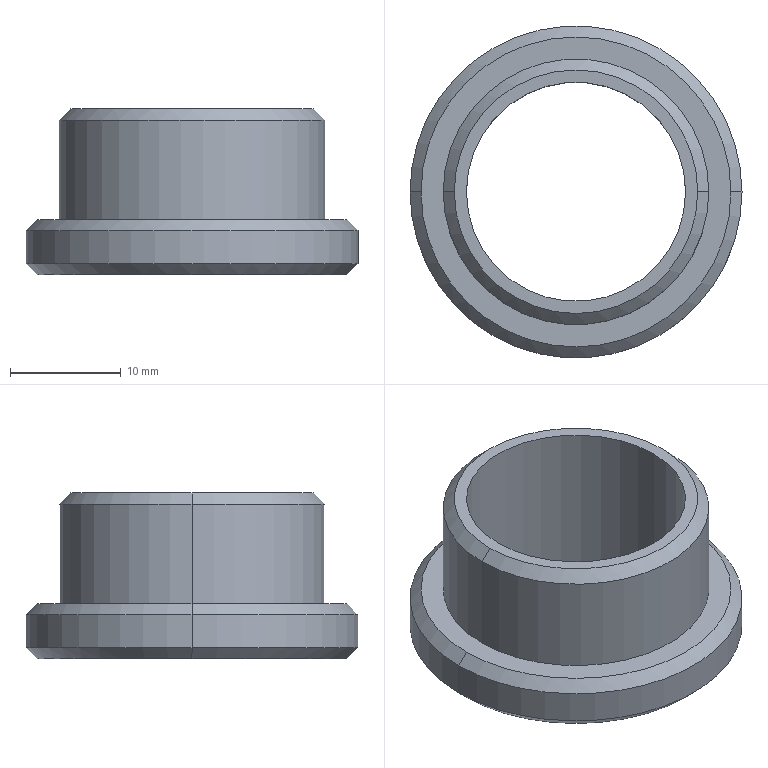Part | SolidWorks | features Chamfer 1, Extrusion 1, ICE 1 | 1 solid | 15 faces | box 30 x 30 x 15 mm | volume 3311 mm3 | cone 6 | cylinder 6 | plane 3 | commonest cylinder face diameters 19.8 x2 24 x2 30 x2
STEP:
#1=CARTESIAN_POINT('',(14.,0.,5.));
#2=VERTEX_POINT('',#1);
#3=CARTESIAN_POINT('',(-14.,0.,5.));
#4=VERTEX_POINT('',#3);
#5=CARTESIAN_POINT('',(0.,0.,5.));
#6=DIRECTION('',(0.,0.,1.));
#7=DIRECTION('',(1.,0.,0.));
#8=AXIS2_PLACEMENT_3D('',#5,#6,#7);
#9=CIRCLE('',#8,14.);
#10=EDGE_CURVE('',#2,#4,#9,.T.);
#11=ORIENTED_EDGE('',*,*,#10,.F.);
#12=CARTESIAN_POINT('',(15.,0.,4.));
#13=VERTEX_POINT('',#12);
#14=CARTESIAN_POINT('',(14.,0.,5.));
#15=DIRECTION('',(0.7071,0.,-0.7071));
#16=VECTOR('',#15,1000.);
#17=LINE('',#14,#16);
#18=EDGE_CURVE('',#2,#13,#17,.T.);
#19=ORIENTED_EDGE('',*,*,#18,.T.);
#20=CARTESIAN_POINT('',(-15.,0.,4.));
#21=VERTEX_POINT('',#20);
#22=CARTESIAN_POINT('',(0.,0.,4.));
#23=DIRECTION('',(0.,0.,-1.));
#24=DIRECTION('',(1.,0.,0.));
#25=AXIS2_PLACEMENT_3D('',#22,#23,#24);
#26=CIRCLE('',#25,15.);
#27=EDGE_CURVE('',#21,#13,#26,.T.);
#28=ORIENTED_EDGE('',*,*,#27,.F.);
#29=CARTESIAN_POINT('',(-14.,0.,5.));
#30=DIRECTION('',(-0.7071,0.,-0.7071));
#31=VECTOR('',#30,1000.);
#32=LINE('',#29,#31);
#33=EDGE_CURVE('',#4,#21,#32,.T.);
#34=ORIENTED_EDGE('',*,*,#33,.F.);
#35=EDGE_LOOP('',(#11,#19,#28,#34));
#36=FACE_OUTER_BOUND('',#35,.T.);
#37=CARTESIAN_POINT('',(0.,0.,5.));
#38=DIRECTION('',(0.,0.,-1.));
#39=DIRECTION('',(-1.,0.,0.));
#40=AXIS2_PLACEMENT_3D('',#37,#38,#39);
#41=CONICAL_SURFACE('',#40,14.,0.7854);
#42=ADVANCED_FACE('',(#36),#41,.T.);
#43=CARTESIAN_POINT('',(-14.,0.,0.));
#44=VERTEX_POINT('',#43);
#45=CARTESIAN_POINT('',(14.,0.,0.));
#46=VERTEX_POINT('',#45);
#47=CARTESIAN_POINT('',(0.,0.,0.));
#48=DIRECTION('',(0.,0.,-1.));
#49=DIRECTION('',(1.,0.,0.));
#50=AXIS2_PLACEMENT_3D('',#47,#48,#49);
#51=CIRCLE('',#50,14.);
#52=EDGE_CURVE('',#44,#46,#51,.T.);
#53=ORIENTED_EDGE('',*,*,#52,.F.);
#54=CARTESIAN_POINT('',(-15.,0.,1.));
#55=VERTEX_POINT('',#54);
#56=CARTESIAN_POINT('',(-15.,0.,1.));
#57=DIRECTION('',(-0.7071,0.,0.7071));
#58=VECTOR('',#57,1000.);
#59=LINE('',#56,#58);
#60=EDGE_CURVE('',#44,#55,#59,.T.);
#61=ORIENTED_EDGE('',*,*,#60,.T.);
#62=CARTESIAN_POINT('',(15.,0.,1.));
#63=VERTEX_POINT('',#62);
#64=CARTESIAN_POINT('',(0.,0.,1.));
#65=DIRECTION('',(0.,0.,1.));
#66=DIRECTION('',(1.,0.,0.));
#67=AXIS2_PLACEMENT_3D('',#64,#65,#66);
#68=CIRCLE('',#67,15.);
#69=EDGE_CURVE('',#63,#55,#68,.T.);
#70=ORIENTED_EDGE('',*,*,#69,.F.);
#71=CARTESIAN_POINT('',(15.,0.,1.));
#72=DIRECTION('',(0.7071,0.,0.7071));
#73=VECTOR('',#72,1000.);
#74=LINE('',#71,#73);
#75=EDGE_CURVE('',#46,#63,#74,.T.);
#76=ORIENTED_EDGE('',*,*,#75,.F.);
#77=EDGE_LOOP('',(#53,#61,#70,#76));
#78=FACE_OUTER_BOUND('',#77,.T.);
#79=CARTESIAN_POINT('',(0.,0.,1.));
#80=DIRECTION('',(0.,0.,1.));
#81=DIRECTION('',(1.,0.,0.));
#82=AXIS2_PLACEMENT_3D('',#79,#80,#81);
#83=CONICAL_SURFACE('',#82,15.,0.7854);
#84=ADVANCED_FACE('',(#78),#83,.T.);
#85=CARTESIAN_POINT('',(11.,0.,15.));
#86=VERTEX_POINT('',#85);
#87=CARTESIAN_POINT('',(-11.,0.,15.));
#88=VERTEX_POINT('',#87);
#89=CARTESIAN_POINT('',(0.,0.,15.));
#90=DIRECTION('',(0.,0.,1.));
#91=DIRECTION('',(1.,0.,0.));
#92=AXIS2_PLACEMENT_3D('',#89,#90,#91);
#93=CIRCLE('',#92,11.);
#94=EDGE_CURVE('',#86,#88,#93,.T.);
#95=ORIENTED_EDGE('',*,*,#94,.F.);
#96=CARTESIAN_POINT('',(12.,0.,14.));
#97=VERTEX_POINT('',#96);
#98=CARTESIAN_POINT('',(11.,0.,15.));
#99=DIRECTION('',(0.7071,0.,-0.7071));
#100=VECTOR('',#99,1000.);
#101=LINE('',#98,#100);
#102=EDGE_CURVE('',#86,#97,#101,.T.);
#103=ORIENTED_EDGE('',*,*,#102,.T.);
#104=CARTESIAN_POINT('',(-12.,0.,14.));
#105=VERTEX_POINT('',#104);
#106=CARTESIAN_POINT('',(0.,0.,14.));
#107=DIRECTION('',(0.,0.,-1.));
#108=DIRECTION('',(1.,0.,0.));
#109=AXIS2_PLACEMENT_3D('',#106,#107,#108);
#110=CIRCLE('',#109,12.);
#111=EDGE_CURVE('',#105,#97,#110,.T.);
#112=ORIENTED_EDGE('',*,*,#111,.F.);
#113=CARTESIAN_POINT('',(-11.,0.,15.));
#114=DIRECTION('',(-0.7071,0.,-0.7071));
#115=VECTOR('',#114,1000.);
#116=LINE('',#113,#115);
#117=EDGE_CURVE('',#88,#105,#116,.T.);
#118=ORIENTED_EDGE('',*,*,#117,.F.);
#119=EDGE_LOOP('',(#95,#103,#112,#118));
#120=FACE_OUTER_BOUND('',#119,.T.);
#121=CARTESIAN_POINT('',(0.,0.,15.));
#122=DIRECTION('',(0.,0.,-1.));
#123=DIRECTION('',(-1.,0.,0.));
#124=AXIS2_PLACEMENT_3D('',#121,#122,#123);
#125=CONICAL_SURFACE('',#124,11.,0.7854);
#126=ADVANCED_FACE('',(#120),#125,.T.);
#127=ORIENTED_EDGE('',*,*,#111,.T.);
#128=CARTESIAN_POINT('',(12.,0.,5.));
#129=VERTEX_POINT('',#128);
#130=CARTESIAN_POINT('',(12.,0.,15.));
#131=DIRECTION('',(0.,0.,-1.));
#132=VECTOR('',#131,1000.);
#133=LINE('',#130,#132);
#134=EDGE_CURVE('',#97,#129,#133,.T.);
#135=ORIENTED_EDGE('',*,*,#134,.T.);
#136=CARTESIAN_POINT('',(-12.,0.,5.));
#137=VERTEX_POINT('',#136);
#138=CARTESIAN_POINT('',(0.,0.,5.));
#139=DIRECTION('',(0.,0.,1.));
#140=DIRECTION('',(1.,0.,0.));
#141=AXIS2_PLACEMENT_3D('',#138,#139,#140);
#142=CIRCLE('',#141,12.);
#143=EDGE_CURVE('',#129,#137,#142,.T.);
#144=ORIENTED_EDGE('',*,*,#143,.T.);
#145=CARTESIAN_POINT('',(-12.,0.,15.));
#146=DIRECTION('',(0.,0.,-1.));
#147=VECTOR('',#146,1000.);
#148=LINE('',#145,#147);
#149=EDGE_CURVE('',#105,#137,#148,.T.);
#150=ORIENTED_EDGE('',*,*,#149,.F.);
#151=EDGE_LOOP('',(#127,#135,#144,#150));
#152=FACE_OUTER_BOUND('',#151,.T.);
#153=CARTESIAN_POINT('',(0.,0.,15.));
#154=DIRECTION('',(0.,0.,-1.));
#155=DIRECTION('',(-1.,0.,0.));
#156=AXIS2_PLACEMENT_3D('',#153,#154,#155);
#157=CYLINDRICAL_SURFACE('',#156,12.);
#158=ADVANCED_FACE('',(#152),#157,.T.);
#159=CARTESIAN_POINT('',(-9.9,0.,15.));
#160=VERTEX_POINT('',#159);
#161=CARTESIAN_POINT('',(9.9,0.,15.));
#162=VERTEX_POINT('',#161);
#163=CARTESIAN_POINT('',(0.,0.,15.));
#164=DIRECTION('',(0.,0.,1.));
#165=DIRECTION('',(1.,0.,0.));
#166=AXIS2_PLACEMENT_3D('',#163,#164,#165);
#167=CIRCLE('',#166,9.9);
#168=EDGE_CURVE('',#160,#162,#167,.T.);
#169=ORIENTED_EDGE('',*,*,#168,.T.);
#170=CARTESIAN_POINT('',(9.9,0.,0.));
#171=VERTEX_POINT('',#170);
#172=CARTESIAN_POINT('',(9.9,0.,5.));
#173=DIRECTION('',(0.,0.,-1.));
#174=VECTOR('',#173,1000.);
#175=LINE('',#172,#174);
#176=EDGE_CURVE('',#162,#171,#175,.T.);
#177=ORIENTED_EDGE('',*,*,#176,.T.);
#178=CARTESIAN_POINT('',(-9.9,0.,0.));
#179=VERTEX_POINT('',#178);
#180=CARTESIAN_POINT('',(0.,0.,0.));
#181=DIRECTION('',(0.,0.,1.));
#182=DIRECTION('',(1.,0.,0.));
#183=AXIS2_PLACEMENT_3D('',#180,#181,#182);
#184=CIRCLE('',#183,9.9);
#185=EDGE_CURVE('',#179,#171,#184,.T.);
#186=ORIENTED_EDGE('',*,*,#185,.F.);
#187=CARTESIAN_POINT('',(-9.9,0.,5.));
#188=DIRECTION('',(0.,0.,-1.));
#189=VECTOR('',#188,1000.);
#190=LINE('',#187,#189);
#191=EDGE_CURVE('',#160,#179,#190,.T.);
#192=ORIENTED_EDGE('',*,*,#191,.F.);
#193=EDGE_LOOP('',(#169,#177,#186,#192));
#194=FACE_OUTER_BOUND('',#193,.T.);
#195=CARTESIAN_POINT('',(0.,0.,5.));
#196=DIRECTION('',(0.,0.,-1.));
#197=DIRECTION('',(-1.,0.,0.));
#198=AXIS2_PLACEMENT_3D('',#195,#196,#197);
#199=CYLINDRICAL_SURFACE('',#198,9.9);
#200=ADVANCED_FACE('',(#194),#199,.F.);
#201=ORIENTED_EDGE('',*,*,#27,.T.);
#202=CARTESIAN_POINT('',(15.,0.,5.));
#203=DIRECTION('',(0.,0.,-1.));
#204=VECTOR('',#203,1000.);
#205=LINE('',#202,#204);
#206=EDGE_CURVE('',#13,#63,#205,.T.);
#207=ORIENTED_EDGE('',*,*,#206,.T.);
#208=ORIENTED_EDGE('',*,*,#69,.T.);
#209=CARTESIAN_POINT('',(-15.,0.,5.));
#210=DIRECTION('',(0.,0.,-1.));
#211=VECTOR('',#210,1000.);
#212=LINE('',#209,#211);
#213=EDGE_CURVE('',#21,#55,#212,.T.);
#214=ORIENTED_EDGE('',*,*,#213,.F.);
#215=EDGE_LOOP('',(#201,#207,#208,#214));
#216=FACE_OUTER_BOUND('',#215,.T.);
#217=CARTESIAN_POINT('',(0.,0.,5.));
#218=DIRECTION('',(0.,0.,-1.));
#219=DIRECTION('',(-1.,0.,0.));
#220=AXIS2_PLACEMENT_3D('',#217,#218,#219);
#221=CYLINDRICAL_SURFACE('',#220,15.);
#222=ADVANCED_FACE('',(#216),#221,.T.);
#223=CARTESIAN_POINT('',(0.,0.,5.));
#224=DIRECTION('',(0.,0.,1.));
#225=DIRECTION('',(1.,0.,0.));
#226=AXIS2_PLACEMENT_3D('',#223,#224,#225);
#227=CIRCLE('',#226,14.);
#228=EDGE_CURVE('',#4,#2,#227,.T.);
#229=ORIENTED_EDGE('',*,*,#228,.T.);
#230=ORIENTED_EDGE('',*,*,#10,.T.);
#231=EDGE_LOOP('',(#229,#230));
#232=FACE_OUTER_BOUND('',#231,.T.);
#233=CARTESIAN_POINT('',(0.,0.,5.));
#234=DIRECTION('',(0.,0.,1.));
#235=DIRECTION('',(1.,0.,0.));
#236=AXIS2_PLACEMENT_3D('',#233,#234,#235);
#237=CIRCLE('',#236,12.);
#238=EDGE_CURVE('',#137,#129,#237,.T.);
#239=ORIENTED_EDGE('',*,*,#238,.F.);
#240=ORIENTED_EDGE('',*,*,#143,.F.);
#241=EDGE_LOOP('',(#239,#240));
#242=FACE_BOUND('',#241,.T.);
#243=CARTESIAN_POINT('',(0.,0.,5.));
#244=DIRECTION('',(0.,0.,1.));
#245=DIRECTION('',(1.,0.,0.));
#246=AXIS2_PLACEMENT_3D('',#243,#244,#245);
#247=PLANE('',#246);
#248=ADVANCED_FACE('',(#232,#242),#247,.T.);
#249=CARTESIAN_POINT('',(0.,0.,0.));
#250=DIRECTION('',(0.,0.,-1.));
#251=DIRECTION('',(1.,0.,0.));
#252=AXIS2_PLACEMENT_3D('',#249,#250,#251);
#253=CIRCLE('',#252,14.);
#254=EDGE_CURVE('',#46,#44,#253,.T.);
#255=ORIENTED_EDGE('',*,*,#254,.T.);
#256=ORIENTED_EDGE('',*,*,#52,.T.);
#257=EDGE_LOOP('',(#255,#256));
#258=FACE_OUTER_BOUND('',#257,.T.);
#259=ORIENTED_EDGE('',*,*,#185,.T.);
#260=CARTESIAN_POINT('',(0.,0.,0.));
#261=DIRECTION('',(0.,0.,1.));
#262=DIRECTION('',(1.,0.,0.));
#263=AXIS2_PLACEMENT_3D('',#260,#261,#262);
#264=CIRCLE('',#263,9.9);
#265=EDGE_CURVE('',#171,#179,#264,.T.);
#266=ORIENTED_EDGE('',*,*,#265,.T.);
#267=EDGE_LOOP('',(#259,#266));
#268=FACE_BOUND('',#267,.T.);
#269=CARTESIAN_POINT('',(0.,0.,0.));
#270=DIRECTION('',(0.,0.,1.));
#271=DIRECTION('',(1.,0.,0.));
#272=AXIS2_PLACEMENT_3D('',#269,#270,#271);
#273=PLANE('',#272);
#274=ADVANCED_FACE('',(#258,#268),#273,.F.);
#275=ORIENTED_EDGE('',*,*,#206,.F.);
#276=CARTESIAN_POINT('',(0.,0.,4.));
#277=DIRECTION('',(0.,0.,-1.));
#278=DIRECTION('',(1.,0.,0.));
#279=AXIS2_PLACEMENT_3D('',#276,#277,#278);
#280=CIRCLE('',#279,15.);
#281=EDGE_CURVE('',#13,#21,#280,.T.);
#282=ORIENTED_EDGE('',*,*,#281,.T.);
#283=ORIENTED_EDGE('',*,*,#213,.T.);
#284=CARTESIAN_POINT('',(0.,0.,1.));
#285=DIRECTION('',(0.,0.,1.));
#286=DIRECTION('',(1.,0.,0.));
#287=AXIS2_PLACEMENT_3D('',#284,#285,#286);
#288=CIRCLE('',#287,15.);
#289=EDGE_CURVE('',#55,#63,#288,.T.);
#290=ORIENTED_EDGE('',*,*,#289,.T.);
#291=EDGE_LOOP('',(#275,#282,#283,#290));
#292=FACE_OUTER_BOUND('',#291,.T.);
#293=CARTESIAN_POINT('',(0.,0.,5.));
#294=DIRECTION('',(0.,0.,-1.));
#295=DIRECTION('',(-1.,0.,0.));
#296=AXIS2_PLACEMENT_3D('',#293,#294,#295);
#297=CYLINDRICAL_SURFACE('',#296,15.);
#298=ADVANCED_FACE('',(#292),#297,.T.);
#299=ORIENTED_EDGE('',*,*,#176,.F.);
#300=CARTESIAN_POINT('',(0.,0.,15.));
#301=DIRECTION('',(0.,0.,1.));
#302=DIRECTION('',(1.,0.,0.));
#303=AXIS2_PLACEMENT_3D('',#300,#301,#302);
#304=CIRCLE('',#303,9.9);
#305=EDGE_CURVE('',#162,#160,#304,.T.);
#306=ORIENTED_EDGE('',*,*,#305,.T.);
#307=ORIENTED_EDGE('',*,*,#191,.T.);
#308=ORIENTED_EDGE('',*,*,#265,.F.);
#309=EDGE_LOOP('',(#299,#306,#307,#308));
#310=FACE_OUTER_BOUND('',#309,.T.);
#311=CARTESIAN_POINT('',(0.,0.,5.));
#312=DIRECTION('',(0.,0.,-1.));
#313=DIRECTION('',(-1.,0.,0.));
#314=AXIS2_PLACEMENT_3D('',#311,#312,#313);
#315=CYLINDRICAL_SURFACE('',#314,9.9);
#316=ADVANCED_FACE('',(#310),#315,.F.);
#317=CARTESIAN_POINT('',(0.,0.,15.));
#318=DIRECTION('',(0.,0.,1.));
#319=DIRECTION('',(1.,0.,0.));
#320=AXIS2_PLACEMENT_3D('',#317,#318,#319);
#321=CIRCLE('',#320,11.);
#322=EDGE_CURVE('',#88,#86,#321,.T.);
#323=ORIENTED_EDGE('',*,*,#322,.T.);
#324=ORIENTED_EDGE('',*,*,#94,.T.);
#325=EDGE_LOOP('',(#323,#324));
#326=FACE_OUTER_BOUND('',#325,.T.);
#327=ORIENTED_EDGE('',*,*,#168,.F.);
#328=ORIENTED_EDGE('',*,*,#305,.F.);
#329=EDGE_LOOP('',(#327,#328));
#330=FACE_BOUND('',#329,.T.);
#331=CARTESIAN_POINT('',(0.,0.,15.));
#332=DIRECTION('',(0.,0.,1.));
#333=DIRECTION('',(1.,0.,0.));
#334=AXIS2_PLACEMENT_3D('',#331,#332,#333);
#335=PLANE('',#334);
#336=ADVANCED_FACE('',(#326,#330),#335,.T.);
#337=ORIENTED_EDGE('',*,*,#134,.F.);
#338=CARTESIAN_POINT('',(0.,0.,14.));
#339=DIRECTION('',(0.,0.,-1.));
#340=DIRECTION('',(1.,0.,0.));
#341=AXIS2_PLACEMENT_3D('',#338,#339,#340);
#342=CIRCLE('',#341,12.);
#343=EDGE_CURVE('',#97,#105,#342,.T.);
#344=ORIENTED_EDGE('',*,*,#343,.T.);
#345=ORIENTED_EDGE('',*,*,#149,.T.);
#346=ORIENTED_EDGE('',*,*,#238,.T.);
#347=EDGE_LOOP('',(#337,#344,#345,#346));
#348=FACE_OUTER_BOUND('',#347,.T.);
#349=CARTESIAN_POINT('',(0.,0.,15.));
#350=DIRECTION('',(0.,0.,-1.));
#351=DIRECTION('',(-1.,0.,0.));
#352=AXIS2_PLACEMENT_3D('',#349,#350,#351);
#353=CYLINDRICAL_SURFACE('',#352,12.);
#354=ADVANCED_FACE('',(#348),#353,.T.);
#355=ORIENTED_EDGE('',*,*,#102,.F.);
#356=ORIENTED_EDGE('',*,*,#322,.F.);
#357=ORIENTED_EDGE('',*,*,#117,.T.);
#358=ORIENTED_EDGE('',*,*,#343,.F.);
#359=EDGE_LOOP('',(#355,#356,#357,#358));
#360=FACE_OUTER_BOUND('',#359,.T.);
#361=CARTESIAN_POINT('',(0.,0.,15.));
#362=DIRECTION('',(0.,0.,-1.));
#363=DIRECTION('',(-1.,0.,0.));
#364=AXIS2_PLACEMENT_3D('',#361,#362,#363);
#365=CONICAL_SURFACE('',#364,11.,0.7854);
#366=ADVANCED_FACE('',(#360),#365,.T.);
#367=ORIENTED_EDGE('',*,*,#60,.F.);
#368=ORIENTED_EDGE('',*,*,#254,.F.);
#369=ORIENTED_EDGE('',*,*,#75,.T.);
#370=ORIENTED_EDGE('',*,*,#289,.F.);
#371=EDGE_LOOP('',(#367,#368,#369,#370));
#372=FACE_OUTER_BOUND('',#371,.T.);
#373=CARTESIAN_POINT('',(0.,0.,1.));
#374=DIRECTION('',(0.,0.,1.));
#375=DIRECTION('',(1.,0.,0.));
#376=AXIS2_PLACEMENT_3D('',#373,#374,#375);
#377=CONICAL_SURFACE('',#376,15.,0.7854);
#378=ADVANCED_FACE('',(#372),#377,.T.);
#379=ORIENTED_EDGE('',*,*,#18,.F.);
#380=ORIENTED_EDGE('',*,*,#228,.F.);
#381=ORIENTED_EDGE('',*,*,#33,.T.);
#382=ORIENTED_EDGE('',*,*,#281,.F.);
#383=EDGE_LOOP('',(#379,#380,#381,#382));
#384=FACE_OUTER_BOUND('',#383,.T.);
#385=CARTESIAN_POINT('',(0.,0.,5.));
#386=DIRECTION('',(0.,0.,-1.));
#387=DIRECTION('',(-1.,0.,0.));
#388=AXIS2_PLACEMENT_3D('',#385,#386,#387);
#389=CONICAL_SURFACE('',#388,14.,0.7854);
#390=ADVANCED_FACE('',(#384),#389,.T.);
#391=CLOSED_SHELL('',(#42,#84,#126,#158,#200,#222,#248,#274,#298,#316,#336,#354,#366,#378,#390));
#392=MANIFOLD_SOLID_BREP('',#391);
#393=CARTESIAN_POINT('',(0.,0.,0.));
#394=DIRECTION('',(0.,0.,1.));
#395=DIRECTION('',(1.,0.,0.));
#396=AXIS2_PLACEMENT_3D('',#393,#394,#395);
#397=(LENGTH_UNIT()NAMED_UNIT(*)SI_UNIT(.MILLI.,.METRE.));
#398=UNCERTAINTY_MEASURE_WITH_UNIT(LENGTH_MEASURE(0.00001),#397,'','');
#399=(NAMED_UNIT(*)PLANE_ANGLE_UNIT()SI_UNIT($,.RADIAN.));
#400=(NAMED_UNIT(*)SI_UNIT($,.STERADIAN.)SOLID_ANGLE_UNIT());
#401=(GEOMETRIC_REPRESENTATION_CONTEXT(3)GLOBAL_UNCERTAINTY_ASSIGNED_CONTEXT((#398))GLOBAL_UNIT_ASSIGNED_CONTEXT((#397,#399,#400))REPRESENTATION_CONTEXT('',''));
#402=ADVANCED_BREP_SHAPE_REPRESENTATION('',(#392,#396),#401);